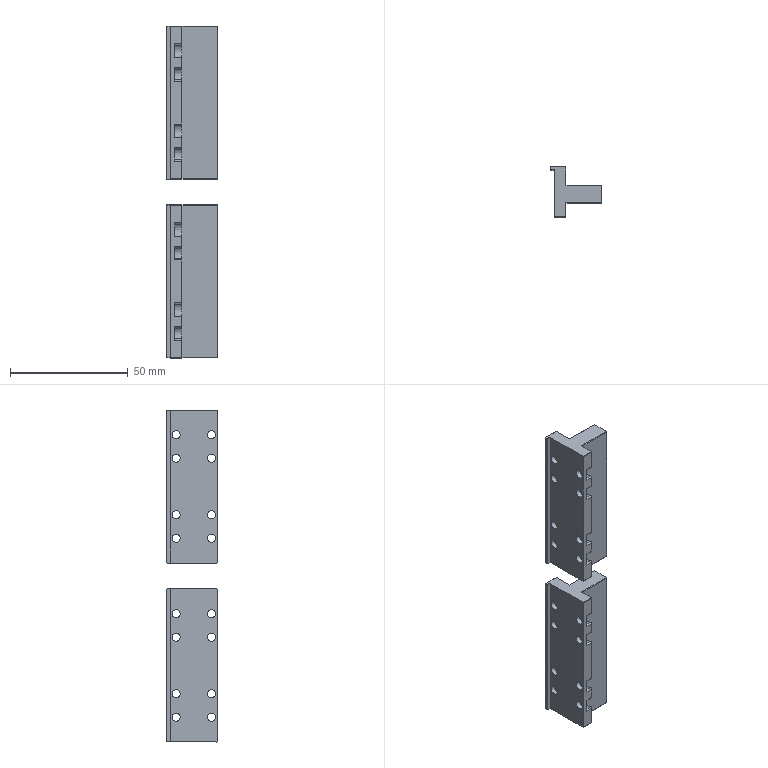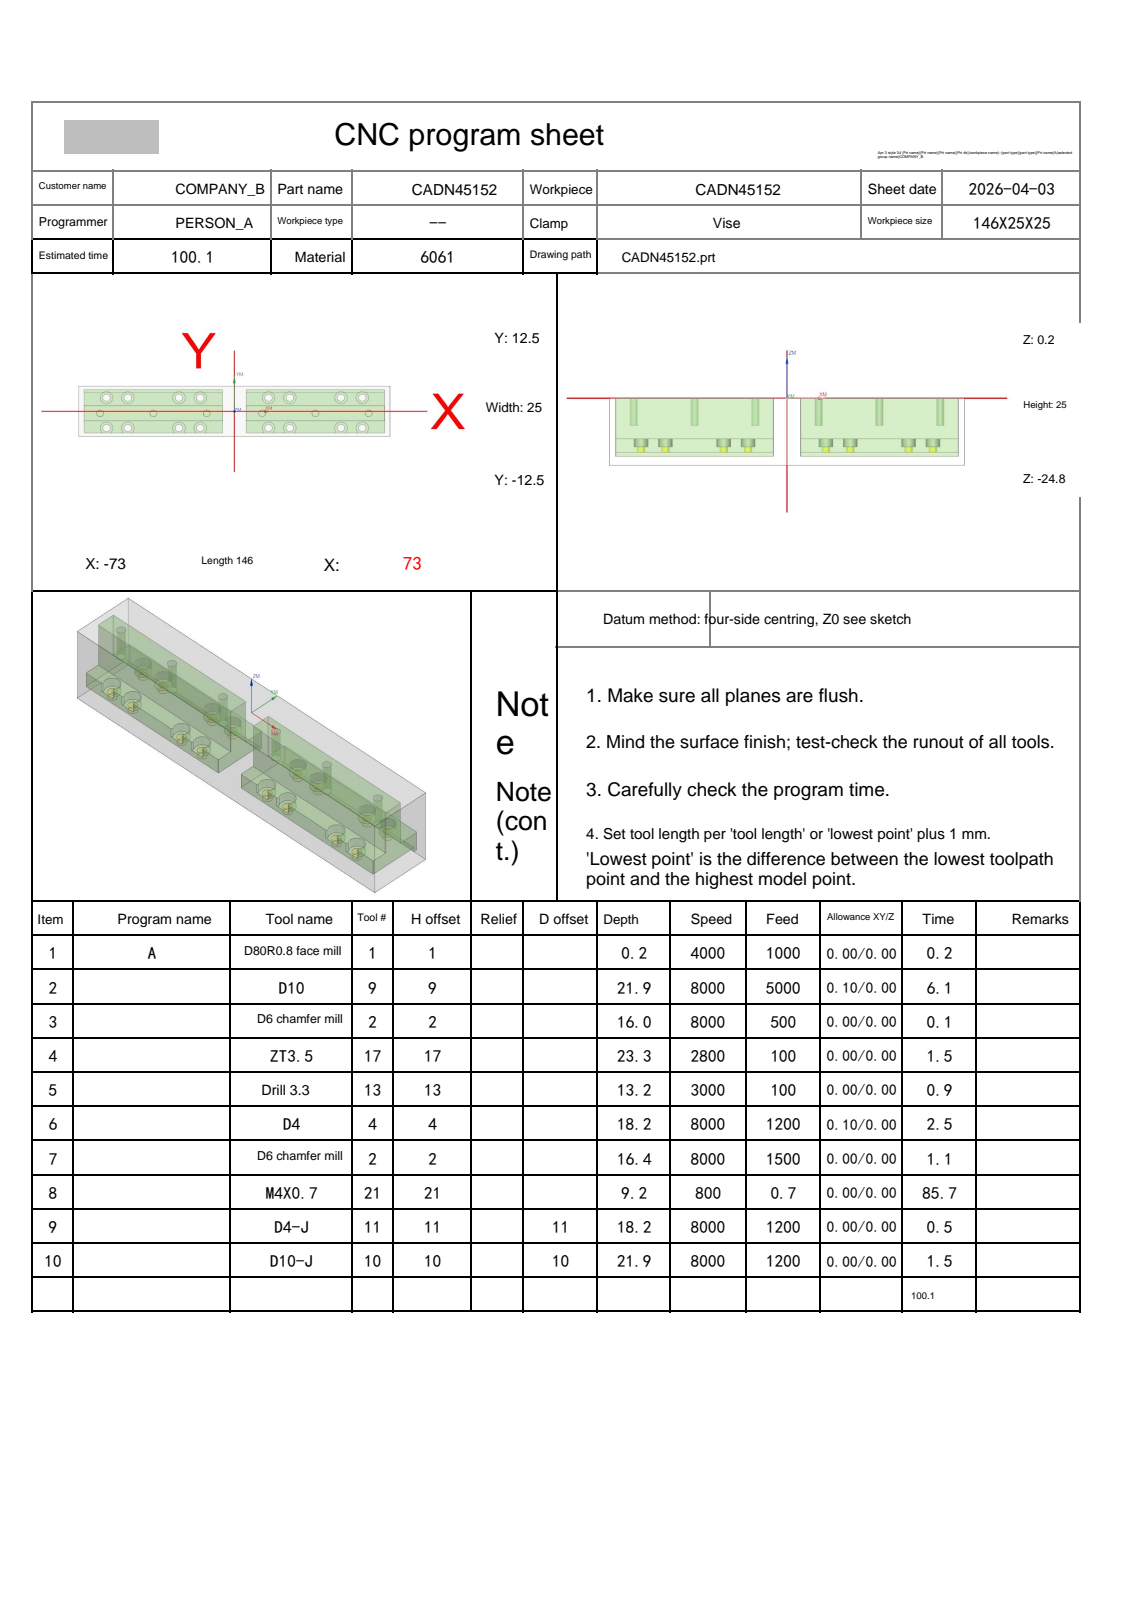NC program | NX | posted by the shop | part box 21.5 x 21.5 x 141 mm
Lines 3869 to 6086 of 7245, first 1796 of 2218 lines:
N3 T02 M06
(D6 chamfer mill  D=6. R=0. H=02 ce=0.00 di=0.10)
G00 G90 G54 X-26. Y-8.25 M03 S8000
G43 H02 Z20.
M08
G98 G81 X-26. Y-8.25 Z-15.8 R-14. F500.
X-16.
Y6.75
X-26.
X-50.
X-60.
X-50. Y-8.25
X-60.
X-63. Y-1. Z-.8 R1.
X-38.
X-13.
X13.
X38.
X63.
X60. Y6.75 Z-15.8 R-14.
X50.
X60. Y-8.25
X50.
X26.
X16.
Y6.75
X26.
G80
G00 Z20.
G91 G28 Z0.0
M05
M09
G91 G28 Z0.0
M01
N4 T17 M06
(ZT3.5 D=3.5 DR_a=118 H=17)
G00 G90 G54 X-50. Y6.75 M03 S2800
G43 H17 Z20.
M08
G98 G83 X-50. Y6.75 Z-23.052 R-14. F100. Q2.
X-60.
Y-8.25
X-50.
X-26.
X-16.
X-26. Y6.75
X-16.
X16.
X26.
X16. Y-8.25
X26.
X50.
X60.
Y6.75
X50.
G80
G00 Z20.
G91 G28 Z0.0
M05
M09
G91 G28 Z0.0
M01
N5 T13 M06
(drill 3.3 D=3.3 DR_a=118 H=13)
G00 G90 G54 X63. Y-1. M03 S3000
G43 H13 Z20.
M08
G98 G83 X63. Y-1. Z-13. R1. F100. Q2.
X38.
X13.
X-13.
X-38.
X-63.
G80
G00 Z20.
G91 G28 Z0.0
M05
M09
G91 G28 Z0.0
M01
N6 T04 M06
(D4  D=4. R=0. H=04 ce=0.10 di=0.10)
G00 G90 G54 X-60. Y-15.75 M03 S6000
G43 H04 Z20.
M08
Z-14.742
G01 Z-15.242 F1200.
Y-11.15
X-59.567
G02 X-59.728 Y-10.25 I2.439 J.9
X-59.261 Y-8.764 I2.6 J0.0
G03 X-59.1 Y-8.25 I-.739 J.514
X-60. Y-7.35 I-.9 J0.0
X-60.9 Y-8.25 I0.0 J-.9
X-60.739 Y-8.764 I.9 J0.0
G02 X-60.272 Y-10.25 I-2.134 J-1.486
X-60.433 Y-11.15 I-2.6 J0.0
G01 X-60.
X-59.567
X-59.589 Y-11.087
Z-14.742
G00 Z-14.5
X-60. Y-15.75
Z-14.983
G01 Z-15.483
Y-11.15
X-59.567
G02 X-59.728 Y-10.25 I2.439 J.9
X-59.261 Y-8.764 I2.6 J0.0
G03 X-59.1 Y-8.25 I-.739 J.514
X-60. Y-7.35 I-.9 J0.0
X-60.9 Y-8.25 I0.0 J-.9
X-60.739 Y-8.764 I.9 J0.0
G02 X-60.272 Y-10.25 I-2.134 J-1.486
X-60.433 Y-11.15 I-2.6 J0.0
G01 X-60.
X-59.567
X-59.589 Y-11.087
Z-14.983
G00 Z-14.742
X-60. Y-15.75
Z-15.225
G01 Z-15.725
Y-11.15
X-59.567
G02 X-59.728 Y-10.25 I2.439 J.9
X-59.261 Y-8.764 I2.6 J0.0
G03 X-59.1 Y-8.25 I-.739 J.514
X-60. Y-7.35 I-.9 J0.0
X-60.9 Y-8.25 I0.0 J-.9
X-60.739 Y-8.764 I.9 J0.0
G02 X-60.272 Y-10.25 I-2.134 J-1.486
X-60.433 Y-11.15 I-2.6 J0.0
G01 X-60.
X-59.567
X-59.589 Y-11.087
Z-15.225
G00 Z-14.983
X-60. Y-15.75
Z-15.467
G01 Z-15.967
Y-11.15
X-59.567
G02 X-59.728 Y-10.25 I2.439 J.9
X-59.261 Y-8.764 I2.6 J0.0
G03 X-59.1 Y-8.25 I-.739 J.514
X-60. Y-7.35 I-.9 J0.0
X-60.9 Y-8.25 I0.0 J-.9
X-60.739 Y-8.764 I.9 J0.0
G02 X-60.272 Y-10.25 I-2.134 J-1.486
X-60.433 Y-11.15 I-2.6 J0.0
G01 X-60.
X-59.567
X-59.589 Y-11.087
Z-15.467
G00 Z-15.225
X-60. Y-15.75
Z-15.708
G01 Z-16.208
Y-11.15
X-59.567
G02 X-59.728 Y-10.25 I2.439 J.9
X-59.261 Y-8.764 I2.6 J0.0
G03 X-59.1 Y-8.25 I-.739 J.514
X-60. Y-7.35 I-.9 J0.0
X-60.9 Y-8.25 I0.0 J-.9
X-60.739 Y-8.764 I.9 J0.0
G02 X-60.272 Y-10.25 I-2.134 J-1.486
X-60.433 Y-11.15 I-2.6 J0.0
G01 X-60.
X-59.567
X-59.589 Y-11.087
Z-15.708
G00 Z-15.467
X-60. Y-15.75
Z-15.95
G01 Z-16.45
Y-11.15
X-59.567
G02 X-59.728 Y-10.25 I2.439 J.9
X-59.261 Y-8.764 I2.6 J0.0
G03 X-59.1 Y-8.25 I-.739 J.514
X-60. Y-7.35 I-.9 J0.0
X-60.9 Y-8.25 I0.0 J-.9
X-60.739 Y-8.764 I.9 J0.0
G02 X-60.272 Y-10.25 I-2.134 J-1.486
X-60.433 Y-11.15 I-2.6 J0.0
G01 X-60.
X-59.567
X-59.589 Y-11.087
Z-15.95
G00 Z-15.708
X-60. Y-15.75
Z-16.192
G01 Z-16.692
Y-11.15
X-59.567
G02 X-59.728 Y-10.25 I2.439 J.9
X-59.261 Y-8.764 I2.6 J0.0
G03 X-59.1 Y-8.25 I-.739 J.514
X-60. Y-7.35 I-.9 J0.0
X-60.9 Y-8.25 I0.0 J-.9
X-60.739 Y-8.764 I.9 J0.0
G02 X-60.272 Y-10.25 I-2.134 J-1.486
X-60.433 Y-11.15 I-2.6 J0.0
G01 X-60.
X-59.567
X-59.589 Y-11.087
Z-16.192
G00 Z-15.95
X-60. Y-15.75
Z-16.433
G01 Z-16.933
Y-11.15
X-59.567
G02 X-59.728 Y-10.25 I2.439 J.9
X-59.261 Y-8.764 I2.6 J0.0
G03 X-59.1 Y-8.25 I-.739 J.514
X-60. Y-7.35 I-.9 J0.0
X-60.9 Y-8.25 I0.0 J-.9
X-60.739 Y-8.764 I.9 J0.0
G02 X-60.272 Y-10.25 I-2.134 J-1.486
X-60.433 Y-11.15 I-2.6 J0.0
G01 X-60.
X-59.567
X-59.589 Y-11.087
Z-16.433
G00 Z-16.192
X-60. Y-15.75
Z-16.675
G01 Z-17.175
Y-11.15
X-59.567
G02 X-59.728 Y-10.25 I2.439 J.9
X-59.261 Y-8.764 I2.6 J0.0
G03 X-59.1 Y-8.25 I-.739 J.514
X-60. Y-7.35 I-.9 J0.0
X-60.9 Y-8.25 I0.0 J-.9
X-60.739 Y-8.764 I.9 J0.0
G02 X-60.272 Y-10.25 I-2.134 J-1.486
X-60.433 Y-11.15 I-2.6 J0.0
G01 X-60.
X-59.567
X-59.589 Y-11.087
Z-16.675
G00 Z-16.433
X-60. Y-15.75
Z-16.917
G01 Z-17.417
Y-11.15
X-59.567
G02 X-59.728 Y-10.25 I2.439 J.9
X-59.261 Y-8.764 I2.6 J0.0
G03 X-59.1 Y-8.25 I-.739 J.514
X-60. Y-7.35 I-.9 J0.0
X-60.9 Y-8.25 I0.0 J-.9
X-60.739 Y-8.764 I.9 J0.0
G02 X-60.272 Y-10.25 I-2.134 J-1.486
X-60.433 Y-11.15 I-2.6 J0.0
G01 X-60.
X-59.567
X-59.589 Y-11.087
Z-16.917
G00 Z-16.675
X-60. Y-15.75
Z-17.158
G01 Z-17.658
Y-11.15
X-59.567
G02 X-59.728 Y-10.25 I2.439 J.9
X-59.261 Y-8.764 I2.6 J0.0
G03 X-59.1 Y-8.25 I-.739 J.514
X-60. Y-7.35 I-.9 J0.0
X-60.9 Y-8.25 I0.0 J-.9
X-60.739 Y-8.764 I.9 J0.0
G02 X-60.272 Y-10.25 I-2.134 J-1.486
X-60.433 Y-11.15 I-2.6 J0.0
G01 X-60.
X-59.567
X-59.589 Y-11.087
Z-17.158
G00 Z-16.917
X-60. Y-15.75
Z-17.4
G01 Z-17.9
Y-11.15
X-59.567
G02 X-59.728 Y-10.25 I2.439 J.9
X-59.261 Y-8.764 I2.6 J0.0
G03 X-59.1 Y-8.25 I-.739 J.514
X-60. Y-7.35 I-.9 J0.0
X-60.9 Y-8.25 I0.0 J-.9
X-60.739 Y-8.764 I.9 J0.0
G02 X-60.272 Y-10.25 I-2.134 J-1.486
X-60.433 Y-11.15 I-2.6 J0.0
G01 X-60.
X-59.567
X-59.589 Y-11.087
Z-17.4
G00 Z20.
X-50. Y-15.75
Z-14.742
G01 Z-15.242
Y-11.15
X-49.567
G02 X-49.728 Y-10.25 I2.439 J.9
X-49.261 Y-8.764 I2.6 J0.0
G03 X-49.1 Y-8.25 I-.739 J.514
X-50. Y-7.35 I-.9 J0.0
X-50.9 Y-8.25 I0.0 J-.9
X-50.739 Y-8.764 I.9 J0.0
G02 X-50.272 Y-10.25 I-2.134 J-1.486
X-50.433 Y-11.15 I-2.6 J0.0
G01 X-50.
X-49.567
X-49.589 Y-11.087
Z-14.742
G00 Z-14.5
X-50. Y-15.75
Z-14.983
G01 Z-15.483
Y-11.15
X-49.567
G02 X-49.728 Y-10.25 I2.439 J.9
X-49.261 Y-8.764 I2.6 J0.0
G03 X-49.1 Y-8.25 I-.739 J.514
X-50. Y-7.35 I-.9 J0.0
X-50.9 Y-8.25 I0.0 J-.9
X-50.739 Y-8.764 I.9 J0.0
G02 X-50.272 Y-10.25 I-2.134 J-1.486
X-50.433 Y-11.15 I-2.6 J0.0
G01 X-50.
X-49.567
X-49.589 Y-11.087
Z-14.983
G00 Z-14.742
X-50. Y-15.75
Z-15.225
G01 Z-15.725
Y-11.15
X-49.567
G02 X-49.728 Y-10.25 I2.439 J.9
X-49.261 Y-8.764 I2.6 J0.0
G03 X-49.1 Y-8.25 I-.739 J.514
X-50. Y-7.35 I-.9 J0.0
X-50.9 Y-8.25 I0.0 J-.9
X-50.739 Y-8.764 I.9 J0.0
G02 X-50.272 Y-10.25 I-2.134 J-1.486
X-50.433 Y-11.15 I-2.6 J0.0
G01 X-50.
X-49.567
X-49.589 Y-11.087
Z-15.225
G00 Z-14.983
X-50. Y-15.75
Z-15.467
G01 Z-15.967
Y-11.15
X-49.567
G02 X-49.728 Y-10.25 I2.439 J.9
X-49.261 Y-8.764 I2.6 J0.0
G03 X-49.1 Y-8.25 I-.739 J.514
X-50. Y-7.35 I-.9 J0.0
X-50.9 Y-8.25 I0.0 J-.9
X-50.739 Y-8.764 I.9 J0.0
G02 X-50.272 Y-10.25 I-2.134 J-1.486
X-50.433 Y-11.15 I-2.6 J0.0
G01 X-50.
X-49.567
X-49.589 Y-11.087
Z-15.467
G00 Z-15.225
X-50. Y-15.75
Z-15.708
G01 Z-16.208
Y-11.15
X-49.567
G02 X-49.728 Y-10.25 I2.439 J.9
X-49.261 Y-8.764 I2.6 J0.0
G03 X-49.1 Y-8.25 I-.739 J.514
X-50. Y-7.35 I-.9 J0.0
X-50.9 Y-8.25 I0.0 J-.9
X-50.739 Y-8.764 I.9 J0.0
G02 X-50.272 Y-10.25 I-2.134 J-1.486
X-50.433 Y-11.15 I-2.6 J0.0
G01 X-50.
X-49.567
X-49.589 Y-11.087
Z-15.708
G00 Z-15.467
X-50. Y-15.75
Z-15.95
G01 Z-16.45
Y-11.15
X-49.567
G02 X-49.728 Y-10.25 I2.439 J.9
X-49.261 Y-8.764 I2.6 J0.0
G03 X-49.1 Y-8.25 I-.739 J.514
X-50. Y-7.35 I-.9 J0.0
X-50.9 Y-8.25 I0.0 J-.9
X-50.739 Y-8.764 I.9 J0.0
G02 X-50.272 Y-10.25 I-2.134 J-1.486
X-50.433 Y-11.15 I-2.6 J0.0
G01 X-50.
X-49.567
X-49.589 Y-11.087
Z-15.95
G00 Z-15.708
X-50. Y-15.75
Z-16.192
G01 Z-16.692
Y-11.15
X-49.567
G02 X-49.728 Y-10.25 I2.439 J.9
X-49.261 Y-8.764 I2.6 J0.0
G03 X-49.1 Y-8.25 I-.739 J.514
X-50. Y-7.35 I-.9 J0.0
X-50.9 Y-8.25 I0.0 J-.9
X-50.739 Y-8.764 I.9 J0.0
G02 X-50.272 Y-10.25 I-2.134 J-1.486
X-50.433 Y-11.15 I-2.6 J0.0
G01 X-50.
X-49.567
X-49.589 Y-11.087
Z-16.192
G00 Z-15.95
X-50. Y-15.75
Z-16.433
G01 Z-16.933
Y-11.15
X-49.567
G02 X-49.728 Y-10.25 I2.439 J.9
X-49.261 Y-8.764 I2.6 J0.0
G03 X-49.1 Y-8.25 I-.739 J.514
X-50. Y-7.35 I-.9 J0.0
X-50.9 Y-8.25 I0.0 J-.9
X-50.739 Y-8.764 I.9 J0.0
G02 X-50.272 Y-10.25 I-2.134 J-1.486
X-50.433 Y-11.15 I-2.6 J0.0
G01 X-50.
X-49.567
X-49.589 Y-11.087
Z-16.433
G00 Z-16.192
X-50. Y-15.75
Z-16.675
G01 Z-17.175
Y-11.15
X-49.567
G02 X-49.728 Y-10.25 I2.439 J.9
X-49.261 Y-8.764 I2.6 J0.0
G03 X-49.1 Y-8.25 I-.739 J.514
X-50. Y-7.35 I-.9 J0.0
X-50.9 Y-8.25 I0.0 J-.9
X-50.739 Y-8.764 I.9 J0.0
G02 X-50.272 Y-10.25 I-2.134 J-1.486
X-50.433 Y-11.15 I-2.6 J0.0
G01 X-50.
X-49.567
X-49.589 Y-11.087
Z-16.675
G00 Z-16.433
X-50. Y-15.75
Z-16.917
G01 Z-17.417
Y-11.15
X-49.567
G02 X-49.728 Y-10.25 I2.439 J.9
X-49.261 Y-8.764 I2.6 J0.0
G03 X-49.1 Y-8.25 I-.739 J.514
X-50. Y-7.35 I-.9 J0.0
X-50.9 Y-8.25 I0.0 J-.9
X-50.739 Y-8.764 I.9 J0.0
G02 X-50.272 Y-10.25 I-2.134 J-1.486
X-50.433 Y-11.15 I-2.6 J0.0
G01 X-50.
X-49.567
X-49.589 Y-11.087
Z-16.917
G00 Z-16.675
X-50. Y-15.75
Z-17.158
G01 Z-17.658
Y-11.15
X-49.567
G02 X-49.728 Y-10.25 I2.439 J.9
X-49.261 Y-8.764 I2.6 J0.0
G03 X-49.1 Y-8.25 I-.739 J.514
X-50. Y-7.35 I-.9 J0.0
X-50.9 Y-8.25 I0.0 J-.9
X-50.739 Y-8.764 I.9 J0.0
G02 X-50.272 Y-10.25 I-2.134 J-1.486
X-50.433 Y-11.15 I-2.6 J0.0
G01 X-50.
X-49.567
X-49.589 Y-11.087
Z-17.158
G00 Z-16.917
X-50. Y-15.75
Z-17.4
G01 Z-17.9
Y-11.15
X-49.567
G02 X-49.728 Y-10.25 I2.439 J.9
X-49.261 Y-8.764 I2.6 J0.0
G03 X-49.1 Y-8.25 I-.739 J.514
X-50. Y-7.35 I-.9 J0.0
X-50.9 Y-8.25 I0.0 J-.9
X-50.739 Y-8.764 I.9 J0.0
G02 X-50.272 Y-10.25 I-2.134 J-1.486
X-50.433 Y-11.15 I-2.6 J0.0
G01 X-50.
X-49.567
X-49.589 Y-11.087
Z-17.4
G00 Z20.
X-26. Y-15.75
Z-14.742
G01 Z-15.242
Y-11.15
X-25.567
G02 X-25.728 Y-10.25 I2.439 J.9
X-25.261 Y-8.764 I2.6 J0.0
G03 X-25.1 Y-8.25 I-.739 J.514
X-26. Y-7.35 I-.9 J0.0
X-26.9 Y-8.25 I0.0 J-.9
X-26.739 Y-8.764 I.9 J0.0
G02 X-26.272 Y-10.25 I-2.134 J-1.486
X-26.433 Y-11.15 I-2.6 J0.0
G01 X-26.
X-25.567
X-25.589 Y-11.087
Z-14.742
G00 Z-14.5
X-26. Y-15.75
Z-14.983
G01 Z-15.483
Y-11.15
X-25.567
G02 X-25.728 Y-10.25 I2.439 J.9
X-25.261 Y-8.764 I2.6 J0.0
G03 X-25.1 Y-8.25 I-.739 J.514
X-26. Y-7.35 I-.9 J0.0
X-26.9 Y-8.25 I0.0 J-.9
X-26.739 Y-8.764 I.9 J0.0
G02 X-26.272 Y-10.25 I-2.134 J-1.486
X-26.433 Y-11.15 I-2.6 J0.0
G01 X-26.
X-25.567
X-25.589 Y-11.087
Z-14.983
G00 Z-14.742
X-26. Y-15.75
Z-15.225
G01 Z-15.725
Y-11.15
X-25.567
G02 X-25.728 Y-10.25 I2.439 J.9
X-25.261 Y-8.764 I2.6 J0.0
G03 X-25.1 Y-8.25 I-.739 J.514
X-26. Y-7.35 I-.9 J0.0
X-26.9 Y-8.25 I0.0 J-.9
X-26.739 Y-8.764 I.9 J0.0
G02 X-26.272 Y-10.25 I-2.134 J-1.486
X-26.433 Y-11.15 I-2.6 J0.0
G01 X-26.
X-25.567
X-25.589 Y-11.087
Z-15.225
G00 Z-14.983
X-26. Y-15.75
Z-15.467
G01 Z-15.967
Y-11.15
X-25.567
G02 X-25.728 Y-10.25 I2.439 J.9
X-25.261 Y-8.764 I2.6 J0.0
G03 X-25.1 Y-8.25 I-.739 J.514
X-26. Y-7.35 I-.9 J0.0
X-26.9 Y-8.25 I0.0 J-.9
X-26.739 Y-8.764 I.9 J0.0
G02 X-26.272 Y-10.25 I-2.134 J-1.486
X-26.433 Y-11.15 I-2.6 J0.0
G01 X-26.
X-25.567
X-25.589 Y-11.087
Z-15.467
G00 Z-15.225
X-26. Y-15.75
Z-15.708
G01 Z-16.208
Y-11.15
X-25.567
G02 X-25.728 Y-10.25 I2.439 J.9
X-25.261 Y-8.764 I2.6 J0.0
G03 X-25.1 Y-8.25 I-.739 J.514
X-26. Y-7.35 I-.9 J0.0
X-26.9 Y-8.25 I0.0 J-.9
X-26.739 Y-8.764 I.9 J0.0
G02 X-26.272 Y-10.25 I-2.134 J-1.486
X-26.433 Y-11.15 I-2.6 J0.0
G01 X-26.
X-25.567
X-25.589 Y-11.087
Z-15.708
G00 Z-15.467
X-26. Y-15.75
Z-15.95
G01 Z-16.45
Y-11.15
X-25.567
G02 X-25.728 Y-10.25 I2.439 J.9
X-25.261 Y-8.764 I2.6 J0.0
G03 X-25.1 Y-8.25 I-.739 J.514
X-26. Y-7.35 I-.9 J0.0
X-26.9 Y-8.25 I0.0 J-.9
X-26.739 Y-8.764 I.9 J0.0
G02 X-26.272 Y-10.25 I-2.134 J-1.486
X-26.433 Y-11.15 I-2.6 J0.0
G01 X-26.
X-25.567
X-25.589 Y-11.087
Z-15.95
G00 Z-15.708
X-26. Y-15.75
Z-16.192
G01 Z-16.692
Y-11.15
X-25.567
G02 X-25.728 Y-10.25 I2.439 J.9
X-25.261 Y-8.764 I2.6 J0.0
G03 X-25.1 Y-8.25 I-.739 J.514
X-26. Y-7.35 I-.9 J0.0
X-26.9 Y-8.25 I0.0 J-.9
X-26.739 Y-8.764 I.9 J0.0
G02 X-26.272 Y-10.25 I-2.134 J-1.486
X-26.433 Y-11.15 I-2.6 J0.0
G01 X-26.
X-25.567
X-25.589 Y-11.087
Z-16.192
G00 Z-15.95
X-26. Y-15.75
Z-16.433
G01 Z-16.933
Y-11.15
X-25.567
G02 X-25.728 Y-10.25 I2.439 J.9
X-25.261 Y-8.764 I2.6 J0.0
G03 X-25.1 Y-8.25 I-.739 J.514
X-26. Y-7.35 I-.9 J0.0
X-26.9 Y-8.25 I0.0 J-.9
X-26.739 Y-8.764 I.9 J0.0
G02 X-26.272 Y-10.25 I-2.134 J-1.486
X-26.433 Y-11.15 I-2.6 J0.0
G01 X-26.
X-25.567
X-25.589 Y-11.087
Z-16.433
G00 Z-16.192
X-26. Y-15.75
Z-16.675
G01 Z-17.175
Y-11.15
X-25.567
G02 X-25.728 Y-10.25 I2.439 J.9
X-25.261 Y-8.764 I2.6 J0.0
G03 X-25.1 Y-8.25 I-.739 J.514
X-26. Y-7.35 I-.9 J0.0
X-26.9 Y-8.25 I0.0 J-.9
X-26.739 Y-8.764 I.9 J0.0
G02 X-26.272 Y-10.25 I-2.134 J-1.486
X-26.433 Y-11.15 I-2.6 J0.0
G01 X-26.
X-25.567
X-25.589 Y-11.087
Z-16.675
G00 Z-16.433
X-26. Y-15.75
Z-16.917
G01 Z-17.417
Y-11.15
X-25.567
G02 X-25.728 Y-10.25 I2.439 J.9
X-25.261 Y-8.764 I2.6 J0.0
G03 X-25.1 Y-8.25 I-.739 J.514
X-26. Y-7.35 I-.9 J0.0
X-26.9 Y-8.25 I0.0 J-.9
X-26.739 Y-8.764 I.9 J0.0
G02 X-26.272 Y-10.25 I-2.134 J-1.486
X-26.433 Y-11.15 I-2.6 J0.0
G01 X-26.
X-25.567
X-25.589 Y-11.087
Z-16.917
G00 Z-16.675
X-26. Y-15.75
Z-17.158
G01 Z-17.658
Y-11.15
X-25.567
G02 X-25.728 Y-10.25 I2.439 J.9
X-25.261 Y-8.764 I2.6 J0.0
G03 X-25.1 Y-8.25 I-.739 J.514
X-26. Y-7.35 I-.9 J0.0
X-26.9 Y-8.25 I0.0 J-.9
X-26.739 Y-8.764 I.9 J0.0
G02 X-26.272 Y-10.25 I-2.134 J-1.486
X-26.433 Y-11.15 I-2.6 J0.0
G01 X-26.
X-25.567
X-25.589 Y-11.087
Z-17.158
G00 Z-16.917
X-26. Y-15.75
Z-17.4
G01 Z-17.9
Y-11.15
X-25.567
G02 X-25.728 Y-10.25 I2.439 J.9
X-25.261 Y-8.764 I2.6 J0.0
G03 X-25.1 Y-8.25 I-.739 J.514
X-26. Y-7.35 I-.9 J0.0
X-26.9 Y-8.25 I0.0 J-.9
X-26.739 Y-8.764 I.9 J0.0
G02 X-26.272 Y-10.25 I-2.134 J-1.486
X-26.433 Y-11.15 I-2.6 J0.0
G01 X-26.
X-25.567
X-25.589 Y-11.087
Z-17.4
G00 Z20.
X-16. Y-15.75
Z-14.742
G01 Z-15.242
Y-11.15
X-15.567
G02 X-15.728 Y-10.25 I2.439 J.9
X-15.261 Y-8.764 I2.6 J0.0
G03 X-15.1 Y-8.25 I-.739 J.514
X-16. Y-7.35 I-.9 J0.0
X-16.9 Y-8.25 I0.0 J-.9
X-16.739 Y-8.764 I.9 J0.0
G02 X-16.272 Y-10.25 I-2.134 J-1.486
X-16.433 Y-11.15 I-2.6 J0.0
G01 X-16.
X-15.567
X-15.589 Y-11.087
Z-14.742
G00 Z-14.5
X-16. Y-15.75
Z-14.983
G01 Z-15.483
Y-11.15
X-15.567
G02 X-15.728 Y-10.25 I2.439 J.9
X-15.261 Y-8.764 I2.6 J0.0
G03 X-15.1 Y-8.25 I-.739 J.514
X-16. Y-7.35 I-.9 J0.0
X-16.9 Y-8.25 I0.0 J-.9
X-16.739 Y-8.764 I.9 J0.0
G02 X-16.272 Y-10.25 I-2.134 J-1.486
X-16.433 Y-11.15 I-2.6 J0.0
G01 X-16.
X-15.567
X-15.589 Y-11.087
Z-14.983
G00 Z-14.742
X-16. Y-15.75
Z-15.225
G01 Z-15.725
Y-11.15
X-15.567
G02 X-15.728 Y-10.25 I2.439 J.9
X-15.261 Y-8.764 I2.6 J0.0
G03 X-15.1 Y-8.25 I-.739 J.514
X-16. Y-7.35 I-.9 J0.0
X-16.9 Y-8.25 I0.0 J-.9
X-16.739 Y-8.764 I.9 J0.0
G02 X-16.272 Y-10.25 I-2.134 J-1.486
X-16.433 Y-11.15 I-2.6 J0.0
G01 X-16.
X-15.567
X-15.589 Y-11.087
Z-15.225
G00 Z-14.983
X-16. Y-15.75
Z-15.467
G01 Z-15.967
Y-11.15
X-15.567
G02 X-15.728 Y-10.25 I2.439 J.9
X-15.261 Y-8.764 I2.6 J0.0
G03 X-15.1 Y-8.25 I-.739 J.514
X-16. Y-7.35 I-.9 J0.0
X-16.9 Y-8.25 I0.0 J-.9
X-16.739 Y-8.764 I.9 J0.0
G02 X-16.272 Y-10.25 I-2.134 J-1.486
X-16.433 Y-11.15 I-2.6 J0.0
G01 X-16.
X-15.567
X-15.589 Y-11.087
Z-15.467
G00 Z-15.225
X-16. Y-15.75
Z-15.708
G01 Z-16.208
Y-11.15
X-15.567
G02 X-15.728 Y-10.25 I2.439 J.9
X-15.261 Y-8.764 I2.6 J0.0
G03 X-15.1 Y-8.25 I-.739 J.514
X-16. Y-7.35 I-.9 J0.0
X-16.9 Y-8.25 I0.0 J-.9
X-16.739 Y-8.764 I.9 J0.0
G02 X-16.272 Y-10.25 I-2.134 J-1.486
X-16.433 Y-11.15 I-2.6 J0.0
G01 X-16.
X-15.567
X-15.589 Y-11.087
Z-15.708
G00 Z-15.467
X-16. Y-15.75
Z-15.95
G01 Z-16.45
Y-11.15
X-15.567
G02 X-15.728 Y-10.25 I2.439 J.9
X-15.261 Y-8.764 I2.6 J0.0
G03 X-15.1 Y-8.25 I-.739 J.514
X-16. Y-7.35 I-.9 J0.0
X-16.9 Y-8.25 I0.0 J-.9
X-16.739 Y-8.764 I.9 J0.0
G02 X-16.272 Y-10.25 I-2.134 J-1.486
X-16.433 Y-11.15 I-2.6 J0.0
G01 X-16.
X-15.567
X-15.589 Y-11.087
Z-15.95
G00 Z-15.708
X-16. Y-15.75
Z-16.192
G01 Z-16.692
Y-11.15
X-15.567
G02 X-15.728 Y-10.25 I2.439 J.9
X-15.261 Y-8.764 I2.6 J0.0
G03 X-15.1 Y-8.25 I-.739 J.514
X-16. Y-7.35 I-.9 J0.0
X-16.9 Y-8.25 I0.0 J-.9
X-16.739 Y-8.764 I.9 J0.0
G02 X-16.272 Y-10.25 I-2.134 J-1.486
X-16.433 Y-11.15 I-2.6 J0.0
G01 X-16.
X-15.567
X-15.589 Y-11.087
Z-16.192
G00 Z-15.95
X-16. Y-15.75
Z-16.433
G01 Z-16.933
Y-11.15
X-15.567
G02 X-15.728 Y-10.25 I2.439 J.9
X-15.261 Y-8.764 I2.6 J0.0
G03 X-15.1 Y-8.25 I-.739 J.514
X-16. Y-7.35 I-.9 J0.0
X-16.9 Y-8.25 I0.0 J-.9
X-16.739 Y-8.764 I.9 J0.0
G02 X-16.272 Y-10.25 I-2.134 J-1.486
X-16.433 Y-11.15 I-2.6 J0.0
G01 X-16.
X-15.567
X-15.589 Y-11.087
Z-16.433
G00 Z-16.192
X-16. Y-15.75
Z-16.675
G01 Z-17.175
Y-11.15
X-15.567
G02 X-15.728 Y-10.25 I2.439 J.9
X-15.261 Y-8.764 I2.6 J0.0
G03 X-15.1 Y-8.25 I-.739 J.514
X-16. Y-7.35 I-.9 J0.0
X-16.9 Y-8.25 I0.0 J-.9
X-16.739 Y-8.764 I.9 J0.0
G02 X-16.272 Y-10.25 I-2.134 J-1.486
X-16.433 Y-11.15 I-2.6 J0.0
G01 X-16.
X-15.567
X-15.589 Y-11.087
Z-16.675
G00 Z-16.433
X-16. Y-15.75
Z-16.917
G01 Z-17.417
Y-11.15
X-15.567
G02 X-15.728 Y-10.25 I2.439 J.9
X-15.261 Y-8.764 I2.6 J0.0
G03 X-15.1 Y-8.25 I-.739 J.514
X-16. Y-7.35 I-.9 J0.0
X-16.9 Y-8.25 I0.0 J-.9
X-16.739 Y-8.764 I.9 J0.0
G02 X-16.272 Y-10.25 I-2.134 J-1.486
X-16.433 Y-11.15 I-2.6 J0.0
G01 X-16.
X-15.567
X-15.589 Y-11.087
Z-16.917
G00 Z-16.675
X-16. Y-15.75
Z-17.158
G01 Z-17.658
Y-11.15
X-15.567
G02 X-15.728 Y-10.25 I2.439 J.9
X-15.261 Y-8.764 I2.6 J0.0
G03 X-15.1 Y-8.25 I-.739 J.514
X-16. Y-7.35 I-.9 J0.0
X-16.9 Y-8.25 I0.0 J-.9
X-16.739 Y-8.764 I.9 J0.0
G02 X-16.272 Y-10.25 I-2.134 J-1.486
X-16.433 Y-11.15 I-2.6 J0.0
G01 X-16.
X-15.567
X-15.589 Y-11.087
Z-17.158
G00 Z-16.917
X-16. Y-15.75
Z-17.4
G01 Z-17.9
Y-11.15
X-15.567
G02 X-15.728 Y-10.25 I2.439 J.9
X-15.261 Y-8.764 I2.6 J0.0
G03 X-15.1 Y-8.25 I-.739 J.514
X-16. Y-7.35 I-.9 J0.0
X-16.9 Y-8.25 I0.0 J-.9
X-16.739 Y-8.764 I.9 J0.0
G02 X-16.272 Y-10.25 I-2.134 J-1.486
X-16.433 Y-11.15 I-2.6 J0.0
G01 X-16.
X-15.567
X-15.589 Y-11.087
Z-17.4
G00 Z20.
X16. Y-15.75
Z-14.742
G01 Z-15.242
Y-11.15
X16.433
G02 X16.272 Y-10.25 I2.439 J.9
X16.739 Y-8.764 I2.6 J0.0
G03 X16.9 Y-8.25 I-.739 J.514
X16. Y-7.35 I-.9 J0.0
X15.1 Y-8.25 I0.0 J-.9
X15.261 Y-8.764 I.9 J0.0
G02 X15.728 Y-10.25 I-2.134 J-1.486
X15.567 Y-11.15 I-2.6 J0.0
G01 X16.
X16.433
X16.411 Y-11.087
Z-14.742
G00 Z-14.5
X16. Y-15.75
Z-14.983
G01 Z-15.483
Y-11.15
X16.433
G02 X16.272 Y-10.25 I2.439 J.9
X16.739 Y-8.764 I2.6 J0.0
G03 X16.9 Y-8.25 I-.739 J.514
X16. Y-7.35 I-.9 J0.0
X15.1 Y-8.25 I0.0 J-.9
X15.261 Y-8.764 I.9 J0.0
G02 X15.728 Y-10.25 I-2.134 J-1.486
X15.567 Y-11.15 I-2.6 J0.0
G01 X16.
X16.433
X16.411 Y-11.087
Z-14.983
G00 Z-14.742
X16. Y-15.75
Z-15.225
G01 Z-15.725
Y-11.15
X16.433
G02 X16.272 Y-10.25 I2.439 J.9
X16.739 Y-8.764 I2.6 J0.0
G03 X16.9 Y-8.25 I-.739 J.514
X16. Y-7.35 I-.9 J0.0
X15.1 Y-8.25 I0.0 J-.9
X15.261 Y-8.764 I.9 J0.0
G02 X15.728 Y-10.25 I-2.134 J-1.486
X15.567 Y-11.15 I-2.6 J0.0
G01 X16.
X16.433
X16.411 Y-11.087
Z-15.225
G00 Z-14.983
X16. Y-15.75
Z-15.467
G01 Z-15.967
Y-11.15
X16.433
G02 X16.272 Y-10.25 I2.439 J.9
X16.739 Y-8.764 I2.6 J0.0
G03 X16.9 Y-8.25 I-.739 J.514
X16. Y-7.35 I-.9 J0.0
X15.1 Y-8.25 I0.0 J-.9
X15.261 Y-8.764 I.9 J0.0
G02 X15.728 Y-10.25 I-2.134 J-1.486
X15.567 Y-11.15 I-2.6 J0.0
G01 X16.
X16.433
X16.411 Y-11.087
Z-15.467
G00 Z-15.225
X16. Y-15.75
Z-15.708
G01 Z-16.208
Y-11.15
X16.433
G02 X16.272 Y-10.25 I2.439 J.9
X16.739 Y-8.764 I2.6 J0.0
G03 X16.9 Y-8.25 I-.739 J.514
X16. Y-7.35 I-.9 J0.0
X15.1 Y-8.25 I0.0 J-.9
X15.261 Y-8.764 I.9 J0.0
G02 X15.728 Y-10.25 I-2.134 J-1.486
X15.567 Y-11.15 I-2.6 J0.0
G01 X16.
X16.433
X16.411 Y-11.087
Z-15.708
G00 Z-15.467
X16. Y-15.75
Z-15.95
G01 Z-16.45
Y-11.15
X16.433
G02 X16.272 Y-10.25 I2.439 J.9
X16.739 Y-8.764 I2.6 J0.0
G03 X16.9 Y-8.25 I-.739 J.514
X16. Y-7.35 I-.9 J0.0
X15.1 Y-8.25 I0.0 J-.9
X15.261 Y-8.764 I.9 J0.0
G02 X15.728 Y-10.25 I-2.134 J-1.486
X15.567 Y-11.15 I-2.6 J0.0
G01 X16.
X16.433
X16.411 Y-11.087
Z-15.95
G00 Z-15.708
X16. Y-15.75
Z-16.192
G01 Z-16.692
Y-11.15
X16.433
G02 X16.272 Y-10.25 I2.439 J.9
X16.739 Y-8.764 I2.6 J0.0
G03 X16.9 Y-8.25 I-.739 J.514
X16. Y-7.35 I-.9 J0.0
X15.1 Y-8.25 I0.0 J-.9
X15.261 Y-8.764 I.9 J0.0
G02 X15.728 Y-10.25 I-2.134 J-1.486
X15.567 Y-11.15 I-2.6 J0.0
G01 X16.
X16.433
X16.411 Y-11.087
Z-16.192
G00 Z-15.95
X16. Y-15.75
Z-16.433
G01 Z-16.933
Y-11.15
X16.433
G02 X16.272 Y-10.25 I2.439 J.9
X16.739 Y-8.764 I2.6 J0.0
G03 X16.9 Y-8.25 I-.739 J.514
X16. Y-7.35 I-.9 J0.0
X15.1 Y-8.25 I0.0 J-.9
X15.261 Y-8.764 I.9 J0.0
G02 X15.728 Y-10.25 I-2.134 J-1.486
X15.567 Y-11.15 I-2.6 J0.0
G01 X16.
X16.433
X16.411 Y-11.087
Z-16.433
G00 Z-16.192
X16. Y-15.75
Z-16.675
G01 Z-17.175
Y-11.15
X16.433
G02 X16.272 Y-10.25 I2.439 J.9
X16.739 Y-8.764 I2.6 J0.0
G03 X16.9 Y-8.25 I-.739 J.514
X16. Y-7.35 I-.9 J0.0
X15.1 Y-8.25 I0.0 J-.9
X15.261 Y-8.764 I.9 J0.0
G02 X15.728 Y-10.25 I-2.134 J-1.486
X15.567 Y-11.15 I-2.6 J0.0
G01 X16.
X16.433
X16.411 Y-11.087
Z-16.675
G00 Z-16.433
X16. Y-15.75
Z-16.917
G01 Z-17.417
Y-11.15
X16.433
G02 X16.272 Y-10.25 I2.439 J.9
X16.739 Y-8.764 I2.6 J0.0
G03 X16.9 Y-8.25 I-.739 J.514
X16. Y-7.35 I-.9 J0.0
X15.1 Y-8.25 I0.0 J-.9
X15.261 Y-8.764 I.9 J0.0
G02 X15.728 Y-10.25 I-2.134 J-1.486
X15.567 Y-11.15 I-2.6 J0.0
G01 X16.
X16.433
X16.411 Y-11.087
Z-16.917
G00 Z-16.675
X16. Y-15.75
Z-17.158
G01 Z-17.658
Y-11.15
X16.433
G02 X16.272 Y-10.25 I2.439 J.9
X16.739 Y-8.764 I2.6 J0.0
G03 X16.9 Y-8.25 I-.739 J.514
X16. Y-7.35 I-.9 J0.0
X15.1 Y-8.25 I0.0 J-.9
X15.261 Y-8.764 I.9 J0.0
G02 X15.728 Y-10.25 I-2.134 J-1.486
X15.567 Y-11.15 I-2.6 J0.0
G01 X16.
X16.433
X16.411 Y-11.087
Z-17.158
G00 Z-16.917
X16. Y-15.75
Z-17.4
G01 Z-17.9
Y-11.15
X16.433
G02 X16.272 Y-10.25 I2.439 J.9
X16.739 Y-8.764 I2.6 J0.0
G03 X16.9 Y-8.25 I-.739 J.514
X16. Y-7.35 I-.9 J0.0
X15.1 Y-8.25 I0.0 J-.9
X15.261 Y-8.764 I.9 J0.0
G02 X15.728 Y-10.25 I-2.134 J-1.486
X15.567 Y-11.15 I-2.6 J0.0
G01 X16.
X16.433
X16.411 Y-11.087
Z-17.4
G00 Z20.
X26. Y-15.75
Z-14.742
G01 Z-15.242
Y-11.15
X26.433
G02 X26.272 Y-10.25 I2.439 J.9
X26.739 Y-8.764 I2.6 J0.0
G03 X26.9 Y-8.25 I-.739 J.514
X26. Y-7.35 I-.9 J0.0
X25.1 Y-8.25 I0.0 J-.9
X25.261 Y-8.764 I.9 J0.0
G02 X25.728 Y-10.25 I-2.134 J-1.486
X25.567 Y-11.15 I-2.6 J0.0
G01 X26.
X26.433
X26.411 Y-11.087
Z-14.742
G00 Z-14.5
X26. Y-15.75
Z-14.983
G01 Z-15.483
Y-11.15
X26.433
G02 X26.272 Y-10.25 I2.439 J.9
X26.739 Y-8.764 I2.6 J0.0
G03 X26.9 Y-8.25 I-.739 J.514
X26. Y-7.35 I-.9 J0.0
X25.1 Y-8.25 I0.0 J-.9
X25.261 Y-8.764 I.9 J0.0
G02 X25.728 Y-10.25 I-2.134 J-1.486
X25.567 Y-11.15 I-2.6 J0.0
G01 X26.
X26.433
X26.411 Y-11.087
Z-14.983
G00 Z-14.742
X26. Y-15.75
Z-15.225
G01 Z-15.725
Y-11.15
X26.433
G02 X26.272 Y-10.25 I2.439 J.9
X26.739 Y-8.764 I2.6 J0.0
G03 X26.9 Y-8.25 I-.739 J.514
X26. Y-7.35 I-.9 J0.0
X25.1 Y-8.25 I0.0 J-.9
X25.261 Y-8.764 I.9 J0.0
G02 X25.728 Y-10.25 I-2.134 J-1.486
X25.567 Y-11.15 I-2.6 J0.0
G01 X26.
X26.433
X26.411 Y-11.087
Z-15.225
G00 Z-14.983
X26. Y-15.75
Z-15.467
G01 Z-15.967
Y-11.15
X26.433
G02 X26.272 Y-10.25 I2.439 J.9
X26.739 Y-8.764 I2.6 J0.0
G03 X26.9 Y-8.25 I-.739 J.514
X26. Y-7.35 I-.9 J0.0
X25.1 Y-8.25 I0.0 J-.9
X25.261 Y-8.764 I.9 J0.0
G02 X25.728 Y-10.25 I-2.134 J-1.486
X25.567 Y-11.15 I-2.6 J0.0
G01 X26.
X26.433
X26.411 Y-11.087
Z-15.467
G00 Z-15.225
X26. Y-15.75
Z-15.708
G01 Z-16.208
Y-11.15
X26.433
G02 X26.272 Y-10.25 I2.439 J.9
X26.739 Y-8.764 I2.6 J0.0
G03 X26.9 Y-8.25 I-.739 J.514
X26. Y-7.35 I-.9 J0.0
X25.1 Y-8.25 I0.0 J-.9
X25.261 Y-8.764 I.9 J0.0
G02 X25.728 Y-10.25 I-2.134 J-1.486
X25.567 Y-11.15 I-2.6 J0.0
G01 X26.
X26.433
X26.411 Y-11.087
Z-15.708
G00 Z-15.467
X26. Y-15.75
Z-15.95
G01 Z-16.45
Y-11.15
X26.433
G02 X26.272 Y-10.25 I2.439 J.9
X26.739 Y-8.764 I2.6 J0.0
G03 X26.9 Y-8.25 I-.739 J.514
X26. Y-7.35 I-.9 J0.0
X25.1 Y-8.25 I0.0 J-.9
X25.261 Y-8.764 I.9 J0.0
G02 X25.728 Y-10.25 I-2.134 J-1.486
X25.567 Y-11.15 I-2.6 J0.0
G01 X26.
X26.433
X26.411 Y-11.087
Z-15.95
G00 Z-15.708
X26. Y-15.75
Z-16.192
G01 Z-16.692
Y-11.15
X26.433
G02 X26.272 Y-10.25 I2.439 J.9
X26.739 Y-8.764 I2.6 J0.0
G03 X26.9 Y-8.25 I-.739 J.514
X26. Y-7.35 I-.9 J0.0
X25.1 Y-8.25 I0.0 J-.9
X25.261 Y-8.764 I.9 J0.0
G02 X25.728 Y-10.25 I-2.134 J-1.486
X25.567 Y-11.15 I-2.6 J0.0
G01 X26.
X26.433
X26.411 Y-11.087
Z-16.192
G00 Z-15.95
X26. Y-15.75
Z-16.433
G01 Z-16.933
Y-11.15
X26.433
G02 X26.272 Y-10.25 I2.439 J.9
X26.739 Y-8.764 I2.6 J0.0
G03 X26.9 Y-8.25 I-.739 J.514
X26. Y-7.35 I-.9 J0.0
X25.1 Y-8.25 I0.0 J-.9
X25.261 Y-8.764 I.9 J0.0
G02 X25.728 Y-10.25 I-2.134 J-1.486
X25.567 Y-11.15 I-2.6 J0.0
G01 X26.
X26.433
X26.411 Y-11.087
Z-16.433
G00 Z-16.192
X26. Y-15.75
Z-16.675
G01 Z-17.175
Y-11.15
X26.433
G02 X26.272 Y-10.25 I2.439 J.9
X26.739 Y-8.764 I2.6 J0.0
G03 X26.9 Y-8.25 I-.739 J.514
X26. Y-7.35 I-.9 J0.0
X25.1 Y-8.25 I0.0 J-.9
X25.261 Y-8.764 I.9 J0.0
G02 X25.728 Y-10.25 I-2.134 J-1.486
X25.567 Y-11.15 I-2.6 J0.0
G01 X26.
X26.433
X26.411 Y-11.087
Z-16.675
G00 Z-16.433
X26. Y-15.75
Z-16.917
G01 Z-17.417
Y-11.15
X26.433
G02 X26.272 Y-10.25 I2.439 J.9
X26.739 Y-8.764 I2.6 J0.0
G03 X26.9 Y-8.25 I-.739 J.514
X26. Y-7.35 I-.9 J0.0
X25.1 Y-8.25 I0.0 J-.9
X25.261 Y-8.764 I.9 J0.0
G02 X25.728 Y-10.25 I-2.134 J-1.486
X25.567 Y-11.15 I-2.6 J0.0
G01 X26.
X26.433
X26.411 Y-11.087
Z-16.917
G00 Z-16.675
X26. Y-15.75
Z-17.158
G01 Z-17.658
Y-11.15
X26.433
G02 X26.272 Y-10.25 I2.439 J.9
X26.739 Y-8.764 I2.6 J0.0
G03 X26.9 Y-8.25 I-.739 J.514
X26. Y-7.35 I-.9 J0.0
X25.1 Y-8.25 I0.0 J-.9
X25.261 Y-8.764 I.9 J0.0
G02 X25.728 Y-10.25 I-2.134 J-1.486
X25.567 Y-11.15 I-2.6 J0.0
G01 X26.
X26.433
X26.411 Y-11.087
Z-17.158
G00 Z-16.917
X26. Y-15.75
Z-17.4
G01 Z-17.9
Y-11.15
X26.433
G02 X26.272 Y-10.25 I2.439 J.9
X26.739 Y-8.764 I2.6 J0.0
G03 X26.9 Y-8.25 I-.739 J.514
X26. Y-7.35 I-.9 J0.0
X25.1 Y-8.25 I0.0 J-.9
X25.261 Y-8.764 I.9 J0.0
G02 X25.728 Y-10.25 I-2.134 J-1.486
X25.567 Y-11.15 I-2.6 J0.0
G01 X26.
X26.433
X26.411 Y-11.087
Z-17.4
G00 Z20.
X60. Y-15.75
Z-14.742
G01 Z-15.242
Y-11.15
X60.433
G02 X60.272 Y-10.25 I2.439 J.9
X60.739 Y-8.764 I2.6 J0.0
G03 X60.9 Y-8.25 I-.739 J.514
X60. Y-7.35 I-.9 J0.0
X59.1 Y-8.25 I0.0 J-.9
X59.261 Y-8.764 I.9 J0.0
G02 X59.728 Y-10.25 I-2.134 J-1.486
X59.567 Y-11.15 I-2.6 J0.0
G01 X60.
X60.433
X60.411 Y-11.087
Z-14.742
G00 Z-14.5
X60. Y-15.75
Z-14.983
G01 Z-15.483
Y-11.15
X60.433
G02 X60.272 Y-10.25 I2.439 J.9
X60.739 Y-8.764 I2.6 J0.0
G03 X60.9 Y-8.25 I-.739 J.514
X60. Y-7.35 I-.9 J0.0
X59.1 Y-8.25 I0.0 J-.9
X59.261 Y-8.764 I.9 J0.0
G02 X59.728 Y-10.25 I-2.134 J-1.486
X59.567 Y-11.15 I-2.6 J0.0
G01 X60.
X60.433
X60.411 Y-11.087
Z-14.983
G00 Z-14.742
X60. Y-15.75
Z-15.225
G01 Z-15.725
Y-11.15
X60.433
G02 X60.272 Y-10.25 I2.439 J.9
X60.739 Y-8.764 I2.6 J0.0
G03 X60.9 Y-8.25 I-.739 J.514
X60. Y-7.35 I-.9 J0.0
X59.1 Y-8.25 I0.0 J-.9
X59.261 Y-8.764 I.9 J0.0
G02 X59.728 Y-10.25 I-2.134 J-1.486
X59.567 Y-11.15 I-2.6 J0.0
G01 X60.
X60.433
X60.411 Y-11.087
Z-15.225
G00 Z-14.983
X60. Y-15.75
Z-15.467
G01 Z-15.967
Y-11.15
X60.433
G02 X60.272 Y-10.25 I2.439 J.9
X60.739 Y-8.764 I2.6 J0.0
G03 X60.9 Y-8.25 I-.739 J.514
X60. Y-7.35 I-.9 J0.0
X59.1 Y-8.25 I0.0 J-.9
X59.261 Y-8.764 I.9 J0.0
G02 X59.728 Y-10.25 I-2.134 J-1.486
X59.567 Y-11.15 I-2.6 J0.0
G01 X60.
X60.433
X60.411 Y-11.087
Z-15.467
G00 Z-15.225
X60. Y-15.75
Z-15.708
G01 Z-16.208
Y-11.15
X60.433
G02 X60.272 Y-10.25 I2.439 J.9
X60.739 Y-8.764 I2.6 J0.0
G03 X60.9 Y-8.25 I-.739 J.514
X60. Y-7.35 I-.9 J0.0
X59.1 Y-8.25 I0.0 J-.9
X59.261 Y-8.764 I.9 J0.0
G02 X59.728 Y-10.25 I-2.134 J-1.486
X59.567 Y-11.15 I-2.6 J0.0
G01 X60.
X60.433
X60.411 Y-11.087
Z-15.708
G00 Z-15.467
X60. Y-15.75
Z-15.95
G01 Z-16.45
Y-11.15
X60.433
G02 X60.272 Y-10.25 I2.439 J.9
X60.739 Y-8.764 I2.6 J0.0
G03 X60.9 Y-8.25 I-.739 J.514
X60. Y-7.35 I-.9 J0.0
X59.1 Y-8.25 I0.0 J-.9
X59.261 Y-8.764 I.9 J0.0
G02 X59.728 Y-10.25 I-2.134 J-1.486
X59.567 Y-11.15 I-2.6 J0.0
G01 X60.
X60.433
X60.411 Y-11.087
Z-15.95
G00 Z-15.708
X60. Y-15.75
Z-16.192
G01 Z-16.692
Y-11.15
X60.433
G02 X60.272 Y-10.25 I2.439 J.9
X60.739 Y-8.764 I2.6 J0.0
G03 X60.9 Y-8.25 I-.739 J.514
X60. Y-7.35 I-.9 J0.0
X59.1 Y-8.25 I0.0 J-.9
X59.261 Y-8.764 I.9 J0.0
G02 X59.728 Y-10.25 I-2.134 J-1.486
X59.567 Y-11.15 I-2.6 J0.0
G01 X60.
X60.433
X60.411 Y-11.087
Z-16.192
G00 Z-15.95
X60. Y-15.75
Z-16.433
G01 Z-16.933
Y-11.15
X60.433
G02 X60.272 Y-10.25 I2.439 J.9
X60.739 Y-8.764 I2.6 J0.0
G03 X60.9 Y-8.25 I-.739 J.514
X60. Y-7.35 I-.9 J0.0
X59.1 Y-8.25 I0.0 J-.9
X59.261 Y-8.764 I.9 J0.0
G02 X59.728 Y-10.25 I-2.134 J-1.486
X59.567 Y-11.15 I-2.6 J0.0
G01 X60.
X60.433
X60.411 Y-11.087
Z-16.433
G00 Z-16.192
X60. Y-15.75
Z-16.675
G01 Z-17.175
Y-11.15
X60.433
G02 X60.272 Y-10.25 I2.439 J.9
X60.739 Y-8.764 I2.6 J0.0
G03 X60.9 Y-8.25 I-.739 J.514
X60. Y-7.35 I-.9 J0.0
X59.1 Y-8.25 I0.0 J-.9
X59.261 Y-8.764 I.9 J0.0
G02 X59.728 Y-10.25 I-2.134 J-1.486
X59.567 Y-11.15 I-2.6 J0.0
G01 X60.
X60.433
X60.411 Y-11.087
Z-16.675
G00 Z-16.433
X60. Y-15.75
Z-16.917
G01 Z-17.417
Y-11.15
X60.433
G02 X60.272 Y-10.25 I2.439 J.9
X60.739 Y-8.764 I2.6 J0.0
G03 X60.9 Y-8.25 I-.739 J.514
X60. Y-7.35 I-.9 J0.0
X59.1 Y-8.25 I0.0 J-.9
X59.261 Y-8.764 I.9 J0.0
G02 X59.728 Y-10.25 I-2.134 J-1.486
X59.567 Y-11.15 I-2.6 J0.0
G01 X60.
X60.433
X60.411 Y-11.087
Z-16.917
G00 Z-16.675
X60. Y-15.75
Z-17.158
G01 Z-17.658
Y-11.15
X60.433
G02 X60.272 Y-10.25 I2.439 J.9
X60.739 Y-8.764 I2.6 J0.0
G03 X60.9 Y-8.25 I-.739 J.514
X60. Y-7.35 I-.9 J0.0
X59.1 Y-8.25 I0.0 J-.9
X59.261 Y-8.764 I.9 J0.0
G02 X59.728 Y-10.25 I-2.134 J-1.486
X59.567 Y-11.15 I-2.6 J0.0
G01 X60.
X60.433
X60.411 Y-11.087
Z-17.158
G00 Z-16.917
X60. Y-15.75
Z-17.4
G01 Z-17.9
Y-11.15
X60.433
G02 X60.272 Y-10.25 I2.439 J.9
X60.739 Y-8.764 I2.6 J0.0
G03 X60.9 Y-8.25 I-.739 J.514
X60. Y-7.35 I-.9 J0.0
X59.1 Y-8.25 I0.0 J-.9
X59.261 Y-8.764 I.9 J0.0
G02 X59.728 Y-10.25 I-2.134 J-1.486
X59.567 Y-11.15 I-2.6 J0.0
G01 X60.
X60.433
X60.411 Y-11.087
Z-17.4
G00 Z20.
X50. Y-15.75
Z-14.742
G01 Z-15.242
Y-11.15
X50.433
G02 X50.272 Y-10.25 I2.439 J.9
X50.739 Y-8.764 I2.6 J0.0
G03 X50.9 Y-8.25 I-.739 J.514
X50. Y-7.35 I-.9 J0.0
X49.1 Y-8.25 I0.0 J-.9
X49.261 Y-8.764 I.9 J0.0
G02 X49.728 Y-10.25 I-2.134 J-1.486
X49.567 Y-11.15 I-2.6 J0.0
G01 X50.
X50.433
X50.411 Y-11.087
Z-14.742
G00 Z-14.5
X50. Y-15.75
Z-14.983
G01 Z-15.483
Y-11.15
X50.433
G02 X50.272 Y-10.25 I2.439 J.9
X50.739 Y-8.764 I2.6 J0.0
G03 X50.9 Y-8.25 I-.739 J.514
X50. Y-7.35 I-.9 J0.0
X49.1 Y-8.25 I0.0 J-.9
X49.261 Y-8.764 I.9 J0.0
G02 X49.728 Y-10.25 I-2.134 J-1.486
X49.567 Y-11.15 I-2.6 J0.0
G01 X50.
X50.433
X50.411 Y-11.087
Z-14.983
G00 Z-14.742
X50. Y-15.75
Z-15.225
G01 Z-15.725
Y-11.15
X50.433
G02 X50.272 Y-10.25 I2.439 J.9
X50.739 Y-8.764 I2.6 J0.0
G03 X50.9 Y-8.25 I-.739 J.514
X50. Y-7.35 I-.9 J0.0
X49.1 Y-8.25 I0.0 J-.9
X49.261 Y-8.764 I.9 J0.0
G02 X49.728 Y-10.25 I-2.134 J-1.486
X49.567 Y-11.15 I-2.6 J0.0
G01 X50.
X50.433
X50.411 Y-11.087
Z-15.225
G00 Z-14.983
X50. Y-15.75
Z-15.467
G01 Z-15.967
Y-11.15
X50.433
G02 X50.272 Y-10.25 I2.439 J.9
X50.739 Y-8.764 I2.6 J0.0
G03 X50.9 Y-8.25 I-.739 J.514
X50. Y-7.35 I-.9 J0.0
X49.1 Y-8.25 I0.0 J-.9
X49.261 Y-8.764 I.9 J0.0
G02 X49.728 Y-10.25 I-2.134 J-1.486
X49.567 Y-11.15 I-2.6 J0.0
G01 X50.
X50.433
X50.411 Y-11.087
Z-15.467
G00 Z-15.225
X50. Y-15.75
Z-15.708
G01 Z-16.208
Y-11.15
X50.433
G02 X50.272 Y-10.25 I2.439 J.9
X50.739 Y-8.764 I2.6 J0.0
G03 X50.9 Y-8.25 I-.739 J.514
X50. Y-7.35 I-.9 J0.0
X49.1 Y-8.25 I0.0 J-.9
X49.261 Y-8.764 I.9 J0.0
G02 X49.728 Y-10.25 I-2.134 J-1.486
X49.567 Y-11.15 I-2.6 J0.0
G01 X50.
X50.433
X50.411 Y-11.087
Z-15.708
G00 Z-15.467
X50. Y-15.75
Z-15.95
G01 Z-16.45
Y-11.15
X50.433
G02 X50.272 Y-10.25 I2.439 J.9
X50.739 Y-8.764 I2.6 J0.0
G03 X50.9 Y-8.25 I-.739 J.514
X50. Y-7.35 I-.9 J0.0
X49.1 Y-8.25 I0.0 J-.9
X49.261 Y-8.764 I.9 J0.0
G02 X49.728 Y-10.25 I-2.134 J-1.486
X49.567 Y-11.15 I-2.6 J0.0
G01 X50.
X50.433
X50.411 Y-11.087
Z-15.95
G00 Z-15.708
X50. Y-15.75
Z-16.192
G01 Z-16.692
Y-11.15
X50.433
G02 X50.272 Y-10.25 I2.439 J.9
X50.739 Y-8.764 I2.6 J0.0
G03 X50.9 Y-8.25 I-.739 J.514
X50. Y-7.35 I-.9 J0.0
X49.1 Y-8.25 I0.0 J-.9
X49.261 Y-8.764 I.9 J0.0
G02 X49.728 Y-10.25 I-2.134 J-1.486
X49.567 Y-11.15 I-2.6 J0.0
G01 X50.
X50.433
X50.411 Y-11.087
Z-16.192
G00 Z-15.95
X50. Y-15.75
Z-16.433
G01 Z-16.933
Y-11.15
X50.433
G02 X50.272 Y-10.25 I2.439 J.9
X50.739 Y-8.764 I2.6 J0.0
G03 X50.9 Y-8.25 I-.739 J.514
X50. Y-7.35 I-.9 J0.0
X49.1 Y-8.25 I0.0 J-.9
X49.261 Y-8.764 I.9 J0.0
G02 X49.728 Y-10.25 I-2.134 J-1.486
X49.567 Y-11.15 I-2.6 J0.0
G01 X50.
X50.433
X50.411 Y-11.087
Z-16.433
G00 Z-16.192
X50. Y-15.75
Z-16.675
G01 Z-17.175
Y-11.15
X50.433
G02 X50.272 Y-10.25 I2.439 J.9
X50.739 Y-8.764 I2.6 J0.0
G03 X50.9 Y-8.25 I-.739 J.514
X50. Y-7.35 I-.9 J0.0
X49.1 Y-8.25 I0.0 J-.9
X49.261 Y-8.764 I.9 J0.0
G02 X49.728 Y-10.25 I-2.134 J-1.486
X49.567 Y-11.15 I-2.6 J0.0
G01 X50.
X50.433
X50.411 Y-11.087
Z-16.675
G00 Z-16.433
X50. Y-15.75
Z-16.917
G01 Z-17.417
Y-11.15
X50.433
G02 X50.272 Y-10.25 I2.439 J.9
X50.739 Y-8.764 I2.6 J0.0
G03 X50.9 Y-8.25 I-.739 J.514
X50. Y-7.35 I-.9 J0.0
X49.1 Y-8.25 I0.0 J-.9
X49.261 Y-8.764 I.9 J0.0
G02 X49.728 Y-10.25 I-2.134 J-1.486
X49.567 Y-11.15 I-2.6 J0.0
G01 X50.
X50.433
X50.411 Y-11.087
Z-16.917
G00 Z-16.675
X50. Y-15.75
Z-17.158
G01 Z-17.658
Y-11.15
X50.433
G02 X50.272 Y-10.25 I2.439 J.9
X50.739 Y-8.764 I2.6 J0.0
G03 X50.9 Y-8.25 I-.739 J.514
X50. Y-7.35 I-.9 J0.0
X49.1 Y-8.25 I0.0 J-.9
X49.261 Y-8.764 I.9 J0.0
G02 X49.728 Y-10.25 I-2.134 J-1.486
X49.567 Y-11.15 I-2.6 J0.0
G01 X50.
X50.433
X50.411 Y-11.087
Z-17.158
G00 Z-16.917
X50. Y-15.75
Z-17.4